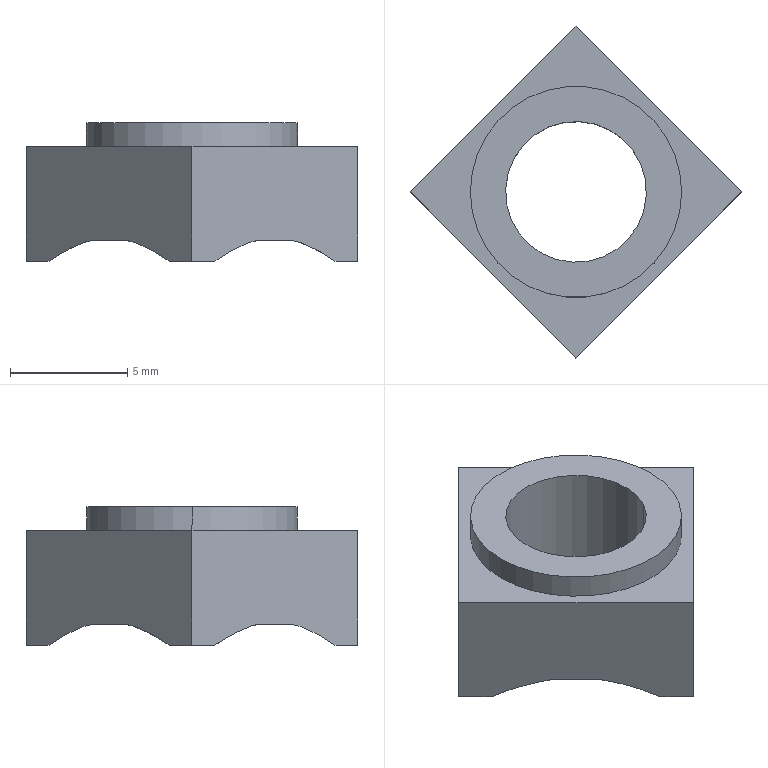Part | STEP file | Q37106 | 1 solid | 20 faces | box 14.142 x 14.142 x 5.9 mm | volume 331.042 mm3 | plane 11 | cone 5 | cylinder 4 | commonest cylinder face diameters 6 x2 9 x2
STEP:
#1=CARTESIAN_POINT('',(2.825,4.246,0.));
#2=VERTEX_POINT('',#1);
#3=CARTESIAN_POINT('',(4.246,2.825,0.));
#4=VERTEX_POINT('',#3);
#5=CARTESIAN_POINT('',(3.536,3.536,0.));
#6=DIRECTION('',(0.7071,-0.7071,0.));
#7=VECTOR('',#6,1.);
#8=LINE('',#5,#7);
#9=EDGE_CURVE('',#2,#4,#8,.T.);
#10=ORIENTED_EDGE('',*,*,#9,.T.);
#11=CARTESIAN_POINT('',(4.476,2.445,0.));
#12=VERTEX_POINT('',#11);
#13=CARTESIAN_POINT('',(0.,0.,0.));
#14=DIRECTION('',(0.,0.,1.));
#15=AXIS2_PLACEMENT_3D('',#13,#14,$);
#16=CIRCLE('',#15,5.1);
#17=EDGE_CURVE('',#12,#4,#16,.T.);
#18=ORIENTED_EDGE('',*,*,#17,.F.);
#19=CARTESIAN_POINT('',(4.246,-2.825,0.));
#20=VERTEX_POINT('',#19);
#21=CARTESIAN_POINT('',(0.,0.,0.));
#22=DIRECTION('',(0.,0.,1.));
#23=AXIS2_PLACEMENT_3D('',#21,#22,$);
#24=CIRCLE('',#23,5.1);
#25=EDGE_CURVE('',#20,#12,#24,.T.);
#26=ORIENTED_EDGE('',*,*,#25,.F.);
#27=CARTESIAN_POINT('',(2.825,-4.246,0.));
#28=VERTEX_POINT('',#27);
#29=CARTESIAN_POINT('',(3.536,-3.536,0.));
#30=DIRECTION('',(-0.7071,-0.7071,0.));
#31=VECTOR('',#30,1.);
#32=LINE('',#29,#31);
#33=EDGE_CURVE('',#20,#28,#32,.T.);
#34=ORIENTED_EDGE('',*,*,#33,.T.);
#35=CARTESIAN_POINT('',(-2.825,-4.246,0.));
#36=VERTEX_POINT('',#35);
#37=CARTESIAN_POINT('',(0.,0.,0.));
#38=DIRECTION('',(0.,0.,1.));
#39=AXIS2_PLACEMENT_3D('',#37,#38,$);
#40=CIRCLE('',#39,5.1);
#41=EDGE_CURVE('',#36,#28,#40,.T.);
#42=ORIENTED_EDGE('',*,*,#41,.F.);
#43=CARTESIAN_POINT('',(-4.246,-2.825,0.));
#44=VERTEX_POINT('',#43);
#45=CARTESIAN_POINT('',(-3.536,-3.536,0.));
#46=DIRECTION('',(0.7071,-0.7071,0.));
#47=VECTOR('',#46,1.);
#48=LINE('',#45,#47);
#49=EDGE_CURVE('',#44,#36,#48,.T.);
#50=ORIENTED_EDGE('',*,*,#49,.F.);
#51=CARTESIAN_POINT('',(-4.476,-2.445,0.));
#52=VERTEX_POINT('',#51);
#53=CARTESIAN_POINT('',(0.,0.,0.));
#54=DIRECTION('',(0.,0.,1.));
#55=AXIS2_PLACEMENT_3D('',#53,#54,$);
#56=CIRCLE('',#55,5.1);
#57=EDGE_CURVE('',#52,#44,#56,.T.);
#58=ORIENTED_EDGE('',*,*,#57,.F.);
#59=CARTESIAN_POINT('',(-4.246,2.825,0.));
#60=VERTEX_POINT('',#59);
#61=CARTESIAN_POINT('',(0.,0.,0.));
#62=DIRECTION('',(0.,0.,1.));
#63=AXIS2_PLACEMENT_3D('',#61,#62,$);
#64=CIRCLE('',#63,5.1);
#65=EDGE_CURVE('',#60,#52,#64,.T.);
#66=ORIENTED_EDGE('',*,*,#65,.F.);
#67=CARTESIAN_POINT('',(-2.825,4.246,0.));
#68=VERTEX_POINT('',#67);
#69=CARTESIAN_POINT('',(-3.536,3.536,0.));
#70=DIRECTION('',(0.7071,0.7071,0.));
#71=VECTOR('',#70,1.);
#72=LINE('',#69,#71);
#73=EDGE_CURVE('',#60,#68,#72,.T.);
#74=ORIENTED_EDGE('',*,*,#73,.T.);
#75=CARTESIAN_POINT('',(0.,0.,0.));
#76=DIRECTION('',(0.,0.,1.));
#77=AXIS2_PLACEMENT_3D('',#75,#76,$);
#78=CIRCLE('',#77,5.1);
#79=EDGE_CURVE('',#2,#68,#78,.T.);
#80=ORIENTED_EDGE('',*,*,#79,.F.);
#81=EDGE_LOOP('',(#10,#18,#26,#34,#42,#50,#58,#66,#74,#80));
#82=FACE_OUTER_BOUND('',#81,.T.);
#83=CARTESIAN_POINT('',(-2.633,1.438,0.));
#84=VERTEX_POINT('',#83);
#85=CARTESIAN_POINT('',(2.633,-1.438,0.));
#86=VERTEX_POINT('',#85);
#87=CARTESIAN_POINT('',(0.,0.,0.));
#88=DIRECTION('',(0.,0.,1.));
#89=AXIS2_PLACEMENT_3D('',#87,#88,$);
#90=CIRCLE('',#89,3.);
#91=EDGE_CURVE('',#84,#86,#90,.T.);
#92=ORIENTED_EDGE('',*,*,#91,.T.);
#93=CARTESIAN_POINT('',(0.,0.,0.));
#94=DIRECTION('',(0.,0.,1.));
#95=AXIS2_PLACEMENT_3D('',#93,#94,$);
#96=CIRCLE('',#95,3.);
#97=EDGE_CURVE('',#86,#84,#96,.T.);
#98=ORIENTED_EDGE('',*,*,#97,.T.);
#99=EDGE_LOOP('',(#92,#98));
#100=FACE_BOUND('',#99,.T.);
#101=CARTESIAN_POINT('',(0.,0.,0.));
#102=DIRECTION('',(0.,0.,1.));
#103=DIRECTION('',(1.,0.,0.));
#104=AXIS2_PLACEMENT_3D('',#101,#102,#103);
#105=PLANE('',#104);
#106=ADVANCED_FACE('',(#82,#100),#105,.F.);
#107=CARTESIAN_POINT('',(-0.9762,6.095,-0.9));
#108=VERTEX_POINT('',#107);
#109=CARTESIAN_POINT('',(-2.825,4.246,0.));
#110=CARTESIAN_POINT('',(-2.43,4.641,-0.09223));
#111=CARTESIAN_POINT('',(-2.013,5.058,-0.2568));
#112=CARTESIAN_POINT('',(-1.552,5.519,-0.4995));
#113=CARTESIAN_POINT('',(-0.9762,6.095,-0.9));
#114=B_SPLINE_CURVE_WITH_KNOTS('',4,(#109,#110,#111,#112,#113),.UNSPECIFIED.,.F.,.U.,(5,5),(0.,42.955),.UNSPECIFIED.);
#115=EDGE_CURVE('',#68,#108,#114,.T.);
#116=ORIENTED_EDGE('',*,*,#115,.T.);
#117=CARTESIAN_POINT('',(0.9762,6.095,-0.9));
#118=VERTEX_POINT('',#117);
#119=CARTESIAN_POINT('',(0.,0.,-0.9));
#120=DIRECTION('',(0.,0.,-1.));
#121=AXIS2_PLACEMENT_3D('',#119,#120,$);
#122=CIRCLE('',#121,6.173);
#123=EDGE_CURVE('',#118,#108,#122,.F.);
#124=ORIENTED_EDGE('',*,*,#123,.F.);
#125=CARTESIAN_POINT('',(2.825,4.246,0.));
#126=CARTESIAN_POINT('',(2.43,4.641,-0.09223));
#127=CARTESIAN_POINT('',(2.013,5.058,-0.2568));
#128=CARTESIAN_POINT('',(1.552,5.519,-0.4995));
#129=CARTESIAN_POINT('',(0.9762,6.095,-0.9));
#130=B_SPLINE_CURVE_WITH_KNOTS('',4,(#125,#126,#127,#128,#129),.UNSPECIFIED.,.F.,.U.,(5,5),(0.,42.955),.UNSPECIFIED.);
#131=EDGE_CURVE('',#2,#118,#130,.T.);
#132=ORIENTED_EDGE('',*,*,#131,.F.);
#133=ORIENTED_EDGE('',*,*,#79,.T.);
#134=EDGE_LOOP('',(#116,#124,#132,#133));
#135=FACE_OUTER_BOUND('',#134,.T.);
#136=CARTESIAN_POINT('',(0.,0.,0.));
#137=DIRECTION('',(0.,0.,-1.));
#138=DIRECTION('',(0.8776,0.4794,0.));
#139=AXIS2_PLACEMENT_3D('',#136,#137,#138);
#140=CONICAL_SURFACE('',#139,5.1,0.8727);
#141=ADVANCED_FACE('',(#135),#140,.F.);
#142=ORIENTED_EDGE('',*,*,#115,.F.);
#143=ORIENTED_EDGE('',*,*,#73,.F.);
#144=CARTESIAN_POINT('',(-6.095,0.9762,-0.9));
#145=VERTEX_POINT('',#144);
#146=CARTESIAN_POINT('',(-4.246,2.825,0.));
#147=CARTESIAN_POINT('',(-4.491,2.58,-0.05731));
#148=CARTESIAN_POINT('',(-4.744,2.327,-0.1403));
#149=CARTESIAN_POINT('',(-5.01,2.061,-0.2515));
#150=CARTESIAN_POINT('',(-5.378,1.693,-0.4379));
#151=CARTESIAN_POINT('',(-5.796,1.275,-0.6993));
#152=CARTESIAN_POINT('',(-5.893,1.178,-0.7617));
#153=CARTESIAN_POINT('',(-5.992,1.079,-0.8284));
#154=CARTESIAN_POINT('',(-6.095,0.9762,-0.9));
#155=B_SPLINE_CURVE_WITH_KNOTS('',5,(#146,#147,#148,#149,#150,#151,#152,#153,#154),.UNSPECIFIED.,.F.,.U.,(6,3,6),(0.,33.361,42.955),.UNSPECIFIED.);
#156=EDGE_CURVE('',#60,#145,#155,.T.);
#157=ORIENTED_EDGE('',*,*,#156,.T.);
#158=CARTESIAN_POINT('',(-7.071,0.,-0.9));
#159=VERTEX_POINT('',#158);
#160=CARTESIAN_POINT('',(-6.583,0.4881,-0.9));
#161=DIRECTION('',(0.7071,0.7071,0.));
#162=VECTOR('',#161,1.);
#163=LINE('',#160,#162);
#164=EDGE_CURVE('',#145,#159,#163,.F.);
#165=ORIENTED_EDGE('',*,*,#164,.T.);
#166=CARTESIAN_POINT('',(-7.071,0.,4.));
#167=VERTEX_POINT('',#166);
#168=CARTESIAN_POINT('',(-7.071,0.,1.55));
#169=DIRECTION('',(0.,0.,1.));
#170=VECTOR('',#169,1.);
#171=LINE('',#168,#170);
#172=EDGE_CURVE('',#159,#167,#171,.T.);
#173=ORIENTED_EDGE('',*,*,#172,.T.);
#174=CARTESIAN_POINT('',(0.,7.071,4.));
#175=VERTEX_POINT('',#174);
#176=CARTESIAN_POINT('',(-3.536,3.536,4.));
#177=DIRECTION('',(0.7071,0.7071,0.));
#178=VECTOR('',#177,1.);
#179=LINE('',#176,#178);
#180=EDGE_CURVE('',#175,#167,#179,.F.);
#181=ORIENTED_EDGE('',*,*,#180,.F.);
#182=CARTESIAN_POINT('',(0.,7.071,-0.9));
#183=VERTEX_POINT('',#182);
#184=CARTESIAN_POINT('',(0.,7.071,1.55));
#185=DIRECTION('',(0.,0.,1.));
#186=VECTOR('',#185,1.);
#187=LINE('',#184,#186);
#188=EDGE_CURVE('',#183,#175,#187,.T.);
#189=ORIENTED_EDGE('',*,*,#188,.F.);
#190=CARTESIAN_POINT('',(-0.4881,6.583,-0.9));
#191=DIRECTION('',(0.7071,0.7071,0.));
#192=VECTOR('',#191,1.);
#193=LINE('',#190,#192);
#194=EDGE_CURVE('',#183,#108,#193,.F.);
#195=ORIENTED_EDGE('',*,*,#194,.T.);
#196=EDGE_LOOP('',(#142,#143,#157,#165,#173,#181,#189,#195));
#197=FACE_OUTER_BOUND('',#196,.T.);
#198=CARTESIAN_POINT('',(-7.071,0.,0.));
#199=DIRECTION('',(0.7071,-0.7071,0.));
#200=DIRECTION('',(0.7071,0.7071,0.));
#201=AXIS2_PLACEMENT_3D('',#198,#199,#200);
#202=PLANE('',#201);
#203=ADVANCED_FACE('',(#197),#202,.F.);
#204=CARTESIAN_POINT('',(-4.573,-2.498,-0.09295));
#205=VERTEX_POINT('',#204);
#206=CARTESIAN_POINT('',(-4.246,-2.825,0.));
#207=CARTESIAN_POINT('',(-4.353,-2.718,-0.02496));
#208=CARTESIAN_POINT('',(-4.461,-2.61,-0.05574));
#209=CARTESIAN_POINT('',(-4.573,-2.498,-0.09295));
#210=B_SPLINE_CURVE_WITH_KNOTS('',3,(#206,#207,#208,#209),.UNSPECIFIED.,.F.,.U.,(4,4),(0.,8.718),.UNSPECIFIED.);
#211=EDGE_CURVE('',#44,#205,#210,.T.);
#212=ORIENTED_EDGE('',*,*,#211,.T.);
#213=CARTESIAN_POINT('',(-6.095,-0.9762,-0.9));
#214=VERTEX_POINT('',#213);
#215=CARTESIAN_POINT('',(-4.573,-2.498,-0.09295));
#216=CARTESIAN_POINT('',(-4.901,-2.17,-0.2026));
#217=CARTESIAN_POINT('',(-5.251,-1.82,-0.3625));
#218=CARTESIAN_POINT('',(-5.636,-1.435,-0.5808));
#219=CARTESIAN_POINT('',(-6.095,-0.9762,-0.9));
#220=B_SPLINE_CURVE_WITH_KNOTS('',4,(#215,#216,#217,#218,#219),.UNSPECIFIED.,.F.,.U.,(5,5),(0.,34.234),.UNSPECIFIED.);
#221=EDGE_CURVE('',#205,#214,#220,.T.);
#222=ORIENTED_EDGE('',*,*,#221,.T.);
#223=CARTESIAN_POINT('',(0.,0.,-0.9));
#224=DIRECTION('',(0.,0.,-1.));
#225=AXIS2_PLACEMENT_3D('',#223,#224,$);
#226=CIRCLE('',#225,6.173);
#227=EDGE_CURVE('',#145,#214,#226,.F.);
#228=ORIENTED_EDGE('',*,*,#227,.F.);
#229=ORIENTED_EDGE('',*,*,#156,.F.);
#230=ORIENTED_EDGE('',*,*,#65,.T.);
#231=ORIENTED_EDGE('',*,*,#57,.T.);
#232=EDGE_LOOP('',(#212,#222,#228,#229,#230,#231));
#233=FACE_OUTER_BOUND('',#232,.T.);
#234=ADVANCED_FACE('',(#233),#140,.F.);
#235=ORIENTED_EDGE('',*,*,#221,.F.);
#236=ORIENTED_EDGE('',*,*,#211,.F.);
#237=ORIENTED_EDGE('',*,*,#49,.T.);
#238=CARTESIAN_POINT('',(-0.9762,-6.095,-0.9));
#239=VERTEX_POINT('',#238);
#240=CARTESIAN_POINT('',(-2.825,-4.246,0.));
#241=CARTESIAN_POINT('',(-2.58,-4.491,-0.05731));
#242=CARTESIAN_POINT('',(-2.327,-4.744,-0.1403));
#243=CARTESIAN_POINT('',(-2.061,-5.01,-0.2515));
#244=CARTESIAN_POINT('',(-1.693,-5.378,-0.4379));
#245=CARTESIAN_POINT('',(-1.275,-5.796,-0.6993));
#246=CARTESIAN_POINT('',(-1.178,-5.893,-0.7617));
#247=CARTESIAN_POINT('',(-1.079,-5.992,-0.8284));
#248=CARTESIAN_POINT('',(-0.9762,-6.095,-0.9));
#249=B_SPLINE_CURVE_WITH_KNOTS('',5,(#240,#241,#242,#243,#244,#245,#246,#247,#248),.UNSPECIFIED.,.F.,.U.,(6,3,6),(0.,33.361,42.955),.UNSPECIFIED.);
#250=EDGE_CURVE('',#36,#239,#249,.T.);
#251=ORIENTED_EDGE('',*,*,#250,.T.);
#252=CARTESIAN_POINT('',(0.,-7.071,-0.9));
#253=VERTEX_POINT('',#252);
#254=CARTESIAN_POINT('',(-0.4881,-6.583,-0.9));
#255=DIRECTION('',(-0.7071,0.7071,0.));
#256=VECTOR('',#255,1.);
#257=LINE('',#254,#256);
#258=EDGE_CURVE('',#239,#253,#257,.F.);
#259=ORIENTED_EDGE('',*,*,#258,.T.);
#260=CARTESIAN_POINT('',(0.,-7.071,4.));
#261=VERTEX_POINT('',#260);
#262=CARTESIAN_POINT('',(0.,-7.071,1.55));
#263=DIRECTION('',(0.,0.,1.));
#264=VECTOR('',#263,1.);
#265=LINE('',#262,#264);
#266=EDGE_CURVE('',#253,#261,#265,.T.);
#267=ORIENTED_EDGE('',*,*,#266,.T.);
#268=CARTESIAN_POINT('',(-3.536,-3.536,4.));
#269=DIRECTION('',(-0.7071,0.7071,0.));
#270=VECTOR('',#269,1.);
#271=LINE('',#268,#270);
#272=EDGE_CURVE('',#167,#261,#271,.F.);
#273=ORIENTED_EDGE('',*,*,#272,.F.);
#274=ORIENTED_EDGE('',*,*,#172,.F.);
#275=CARTESIAN_POINT('',(-6.583,-0.4881,-0.9));
#276=DIRECTION('',(-0.7071,0.7071,0.));
#277=VECTOR('',#276,1.);
#278=LINE('',#275,#277);
#279=EDGE_CURVE('',#159,#214,#278,.F.);
#280=ORIENTED_EDGE('',*,*,#279,.T.);
#281=EDGE_LOOP('',(#235,#236,#237,#251,#259,#267,#273,#274,#280));
#282=FACE_OUTER_BOUND('',#281,.T.);
#283=CARTESIAN_POINT('',(0.,-7.071,0.));
#284=DIRECTION('',(0.7071,0.7071,0.));
#285=DIRECTION('',(-0.7071,0.7071,0.));
#286=AXIS2_PLACEMENT_3D('',#283,#284,#285);
#287=PLANE('',#286);
#288=ADVANCED_FACE('',(#282),#287,.F.);
#289=CARTESIAN_POINT('',(0.9762,-6.095,-0.9));
#290=VERTEX_POINT('',#289);
#291=CARTESIAN_POINT('',(2.825,-4.246,0.));
#292=CARTESIAN_POINT('',(2.43,-4.641,-0.09223));
#293=CARTESIAN_POINT('',(2.013,-5.058,-0.2568));
#294=CARTESIAN_POINT('',(1.552,-5.519,-0.4995));
#295=CARTESIAN_POINT('',(0.9762,-6.095,-0.9));
#296=B_SPLINE_CURVE_WITH_KNOTS('',4,(#291,#292,#293,#294,#295),.UNSPECIFIED.,.F.,.U.,(5,5),(0.,42.955),.UNSPECIFIED.);
#297=EDGE_CURVE('',#28,#290,#296,.T.);
#298=ORIENTED_EDGE('',*,*,#297,.T.);
#299=CARTESIAN_POINT('',(0.,0.,-0.9));
#300=DIRECTION('',(0.,0.,-1.));
#301=AXIS2_PLACEMENT_3D('',#299,#300,$);
#302=CIRCLE('',#301,6.173);
#303=EDGE_CURVE('',#239,#290,#302,.F.);
#304=ORIENTED_EDGE('',*,*,#303,.F.);
#305=ORIENTED_EDGE('',*,*,#250,.F.);
#306=ORIENTED_EDGE('',*,*,#41,.T.);
#307=EDGE_LOOP('',(#298,#304,#305,#306));
#308=FACE_OUTER_BOUND('',#307,.T.);
#309=ADVANCED_FACE('',(#308),#140,.F.);
#310=ORIENTED_EDGE('',*,*,#297,.F.);
#311=ORIENTED_EDGE('',*,*,#33,.F.);
#312=CARTESIAN_POINT('',(6.095,-0.9762,-0.9));
#313=VERTEX_POINT('',#312);
#314=CARTESIAN_POINT('',(4.246,-2.825,0.));
#315=CARTESIAN_POINT('',(4.491,-2.58,-0.05731));
#316=CARTESIAN_POINT('',(4.744,-2.327,-0.1403));
#317=CARTESIAN_POINT('',(5.01,-2.061,-0.2515));
#318=CARTESIAN_POINT('',(5.378,-1.693,-0.4379));
#319=CARTESIAN_POINT('',(5.796,-1.275,-0.6993));
#320=CARTESIAN_POINT('',(5.893,-1.178,-0.7617));
#321=CARTESIAN_POINT('',(5.992,-1.079,-0.8284));
#322=CARTESIAN_POINT('',(6.095,-0.9762,-0.9));
#323=B_SPLINE_CURVE_WITH_KNOTS('',5,(#314,#315,#316,#317,#318,#319,#320,#321,#322),.UNSPECIFIED.,.F.,.U.,(6,3,6),(0.,33.361,42.955),.UNSPECIFIED.);
#324=EDGE_CURVE('',#20,#313,#323,.T.);
#325=ORIENTED_EDGE('',*,*,#324,.T.);
#326=CARTESIAN_POINT('',(7.071,0.,-0.9));
#327=VERTEX_POINT('',#326);
#328=CARTESIAN_POINT('',(6.583,-0.4881,-0.9));
#329=DIRECTION('',(-0.7071,-0.7071,0.));
#330=VECTOR('',#329,1.);
#331=LINE('',#328,#330);
#332=EDGE_CURVE('',#313,#327,#331,.F.);
#333=ORIENTED_EDGE('',*,*,#332,.T.);
#334=CARTESIAN_POINT('',(7.071,0.,4.));
#335=VERTEX_POINT('',#334);
#336=CARTESIAN_POINT('',(7.071,0.,1.55));
#337=DIRECTION('',(0.,0.,1.));
#338=VECTOR('',#337,1.);
#339=LINE('',#336,#338);
#340=EDGE_CURVE('',#327,#335,#339,.T.);
#341=ORIENTED_EDGE('',*,*,#340,.T.);
#342=CARTESIAN_POINT('',(3.536,-3.536,4.));
#343=DIRECTION('',(-0.7071,-0.7071,0.));
#344=VECTOR('',#343,1.);
#345=LINE('',#342,#344);
#346=EDGE_CURVE('',#261,#335,#345,.F.);
#347=ORIENTED_EDGE('',*,*,#346,.F.);
#348=ORIENTED_EDGE('',*,*,#266,.F.);
#349=CARTESIAN_POINT('',(0.4881,-6.583,-0.9));
#350=DIRECTION('',(-0.7071,-0.7071,0.));
#351=VECTOR('',#350,1.);
#352=LINE('',#349,#351);
#353=EDGE_CURVE('',#253,#290,#352,.F.);
#354=ORIENTED_EDGE('',*,*,#353,.T.);
#355=EDGE_LOOP('',(#310,#311,#325,#333,#341,#347,#348,#354));
#356=FACE_OUTER_BOUND('',#355,.T.);
#357=CARTESIAN_POINT('',(7.071,0.,0.));
#358=DIRECTION('',(-0.7071,0.7071,0.));
#359=DIRECTION('',(-0.7071,-0.7071,0.));
#360=AXIS2_PLACEMENT_3D('',#357,#358,#359);
#361=PLANE('',#360);
#362=ADVANCED_FACE('',(#356),#361,.F.);
#363=CARTESIAN_POINT('',(4.573,2.498,-0.09295));
#364=VERTEX_POINT('',#363);
#365=CARTESIAN_POINT('',(6.095,0.9762,-0.9));
#366=VERTEX_POINT('',#365);
#367=CARTESIAN_POINT('',(4.573,2.498,-0.09295));
#368=CARTESIAN_POINT('',(4.901,2.17,-0.2026));
#369=CARTESIAN_POINT('',(5.251,1.82,-0.3625));
#370=CARTESIAN_POINT('',(5.636,1.435,-0.5808));
#371=CARTESIAN_POINT('',(6.095,0.9762,-0.9));
#372=B_SPLINE_CURVE_WITH_KNOTS('',4,(#367,#368,#369,#370,#371),.UNSPECIFIED.,.F.,.U.,(5,5),(0.,34.234),.UNSPECIFIED.);
#373=EDGE_CURVE('',#364,#366,#372,.T.);
#374=ORIENTED_EDGE('',*,*,#373,.T.);
#375=CARTESIAN_POINT('',(0.,0.,-0.9));
#376=DIRECTION('',(0.,0.,-1.));
#377=AXIS2_PLACEMENT_3D('',#375,#376,$);
#378=CIRCLE('',#377,6.173);
#379=EDGE_CURVE('',#313,#366,#378,.F.);
#380=ORIENTED_EDGE('',*,*,#379,.F.);
#381=ORIENTED_EDGE('',*,*,#324,.F.);
#382=ORIENTED_EDGE('',*,*,#25,.T.);
#383=CARTESIAN_POINT('',(5.014,2.739,-0.5143));
#384=DIRECTION('',(0.6723,0.3673,-0.6428));
#385=VECTOR('',#384,1.);
#386=LINE('',#383,#385);
#387=EDGE_CURVE('',#12,#364,#386,.T.);
#388=ORIENTED_EDGE('',*,*,#387,.T.);
#389=EDGE_LOOP('',(#374,#380,#381,#382,#388));
#390=FACE_OUTER_BOUND('',#389,.T.);
#391=ADVANCED_FACE('',(#390),#140,.F.);
#392=CARTESIAN_POINT('',(4.246,2.825,0.));
#393=CARTESIAN_POINT('',(4.353,2.718,-0.02496));
#394=CARTESIAN_POINT('',(4.461,2.61,-0.05574));
#395=CARTESIAN_POINT('',(4.573,2.498,-0.09295));
#396=B_SPLINE_CURVE_WITH_KNOTS('',3,(#392,#393,#394,#395),.UNSPECIFIED.,.F.,.U.,(4,4),(0.,8.718),.UNSPECIFIED.);
#397=EDGE_CURVE('',#4,#364,#396,.T.);
#398=ORIENTED_EDGE('',*,*,#397,.T.);
#399=ORIENTED_EDGE('',*,*,#387,.F.);
#400=ORIENTED_EDGE('',*,*,#17,.T.);
#401=EDGE_LOOP('',(#398,#399,#400));
#402=FACE_OUTER_BOUND('',#401,.T.);
#403=ADVANCED_FACE('',(#402),#140,.F.);
#404=ORIENTED_EDGE('',*,*,#373,.F.);
#405=ORIENTED_EDGE('',*,*,#397,.F.);
#406=ORIENTED_EDGE('',*,*,#9,.F.);
#407=ORIENTED_EDGE('',*,*,#131,.T.);
#408=CARTESIAN_POINT('',(0.4881,6.583,-0.9));
#409=DIRECTION('',(0.7071,-0.7071,0.));
#410=VECTOR('',#409,1.);
#411=LINE('',#408,#410);
#412=EDGE_CURVE('',#118,#183,#411,.F.);
#413=ORIENTED_EDGE('',*,*,#412,.T.);
#414=ORIENTED_EDGE('',*,*,#188,.T.);
#415=CARTESIAN_POINT('',(3.536,3.536,4.));
#416=DIRECTION('',(0.7071,-0.7071,0.));
#417=VECTOR('',#416,1.);
#418=LINE('',#415,#417);
#419=EDGE_CURVE('',#335,#175,#418,.F.);
#420=ORIENTED_EDGE('',*,*,#419,.F.);
#421=ORIENTED_EDGE('',*,*,#340,.F.);
#422=CARTESIAN_POINT('',(6.583,0.4881,-0.9));
#423=DIRECTION('',(0.7071,-0.7071,0.));
#424=VECTOR('',#423,1.);
#425=LINE('',#422,#424);
#426=EDGE_CURVE('',#327,#366,#425,.F.);
#427=ORIENTED_EDGE('',*,*,#426,.T.);
#428=EDGE_LOOP('',(#404,#405,#406,#407,#413,#414,#420,#421,#427));
#429=FACE_OUTER_BOUND('',#428,.T.);
#430=CARTESIAN_POINT('',(0.,7.071,0.));
#431=DIRECTION('',(-0.7071,-0.7071,0.));
#432=DIRECTION('',(0.7071,-0.7071,0.));
#433=AXIS2_PLACEMENT_3D('',#430,#431,#432);
#434=PLANE('',#433);
#435=ADVANCED_FACE('',(#429),#434,.F.);
#436=ORIENTED_EDGE('',*,*,#97,.F.);
#437=CARTESIAN_POINT('',(2.633,-1.438,5.));
#438=VERTEX_POINT('',#437);
#439=CARTESIAN_POINT('',(2.633,-1.438,2.05));
#440=DIRECTION('',(0.,0.,-1.));
#441=VECTOR('',#440,1.);
#442=LINE('',#439,#441);
#443=EDGE_CURVE('',#86,#438,#442,.F.);
#444=ORIENTED_EDGE('',*,*,#443,.T.);
#445=CARTESIAN_POINT('',(-2.633,1.438,5.));
#446=VERTEX_POINT('',#445);
#447=CARTESIAN_POINT('',(0.,0.,5.));
#448=DIRECTION('',(0.,0.,-1.));
#449=AXIS2_PLACEMENT_3D('',#447,#448,$);
#450=CIRCLE('',#449,3.);
#451=EDGE_CURVE('',#438,#446,#450,.F.);
#452=ORIENTED_EDGE('',*,*,#451,.T.);
#453=CARTESIAN_POINT('',(-2.633,1.438,2.05));
#454=DIRECTION('',(0.,0.,-1.));
#455=VECTOR('',#454,1.);
#456=LINE('',#453,#455);
#457=EDGE_CURVE('',#84,#446,#456,.F.);
#458=ORIENTED_EDGE('',*,*,#457,.F.);
#459=EDGE_LOOP('',(#436,#444,#452,#458));
#460=FACE_OUTER_BOUND('',#459,.T.);
#461=CARTESIAN_POINT('',(0.,0.,4.7));
#462=DIRECTION('',(0.,0.,-1.));
#463=DIRECTION('',(0.8776,-0.4794,0.));
#464=AXIS2_PLACEMENT_3D('',#461,#462,#463);
#465=CYLINDRICAL_SURFACE('',#464,3.);
#466=ADVANCED_FACE('',(#460),#465,.F.);
#467=ORIENTED_EDGE('',*,*,#91,.F.);
#468=ORIENTED_EDGE('',*,*,#457,.T.);
#469=CARTESIAN_POINT('',(0.,0.,5.));
#470=DIRECTION('',(0.,0.,-1.));
#471=AXIS2_PLACEMENT_3D('',#469,#470,$);
#472=CIRCLE('',#471,3.);
#473=EDGE_CURVE('',#446,#438,#472,.F.);
#474=ORIENTED_EDGE('',*,*,#473,.T.);
#475=ORIENTED_EDGE('',*,*,#443,.F.);
#476=EDGE_LOOP('',(#467,#468,#474,#475));
#477=FACE_OUTER_BOUND('',#476,.T.);
#478=ADVANCED_FACE('',(#477),#465,.F.);
#479=ORIENTED_EDGE('',*,*,#123,.T.);
#480=ORIENTED_EDGE('',*,*,#194,.F.);
#481=ORIENTED_EDGE('',*,*,#412,.F.);
#482=EDGE_LOOP('',(#479,#480,#481));
#483=FACE_OUTER_BOUND('',#482,.T.);
#484=CARTESIAN_POINT('',(0.,0.,-0.9));
#485=DIRECTION('',(0.,0.,1.));
#486=DIRECTION('',(1.,0.,0.));
#487=AXIS2_PLACEMENT_3D('',#484,#485,#486);
#488=PLANE('',#487);
#489=ADVANCED_FACE('',(#483),#488,.F.);
#490=ORIENTED_EDGE('',*,*,#227,.T.);
#491=ORIENTED_EDGE('',*,*,#279,.F.);
#492=ORIENTED_EDGE('',*,*,#164,.F.);
#493=EDGE_LOOP('',(#490,#491,#492));
#494=FACE_OUTER_BOUND('',#493,.T.);
#495=ADVANCED_FACE('',(#494),#488,.F.);
#496=ORIENTED_EDGE('',*,*,#272,.T.);
#497=ORIENTED_EDGE('',*,*,#346,.T.);
#498=ORIENTED_EDGE('',*,*,#419,.T.);
#499=ORIENTED_EDGE('',*,*,#180,.T.);
#500=EDGE_LOOP('',(#496,#497,#498,#499));
#501=FACE_OUTER_BOUND('',#500,.T.);
#502=CARTESIAN_POINT('',(4.5,0.,4.));
#503=VERTEX_POINT('',#502);
#504=CARTESIAN_POINT('',(-4.5,0.,4.));
#505=VERTEX_POINT('',#504);
#506=CARTESIAN_POINT('',(0.,0.,4.));
#507=DIRECTION('',(0.,0.,1.));
#508=AXIS2_PLACEMENT_3D('',#506,#507,$);
#509=CIRCLE('',#508,4.5);
#510=EDGE_CURVE('',#503,#505,#509,.T.);
#511=ORIENTED_EDGE('',*,*,#510,.F.);
#512=CARTESIAN_POINT('',(0.,0.,4.));
#513=DIRECTION('',(0.,0.,1.));
#514=AXIS2_PLACEMENT_3D('',#512,#513,$);
#515=CIRCLE('',#514,4.5);
#516=EDGE_CURVE('',#505,#503,#515,.T.);
#517=ORIENTED_EDGE('',*,*,#516,.F.);
#518=EDGE_LOOP('',(#511,#517));
#519=FACE_BOUND('',#518,.T.);
#520=CARTESIAN_POINT('',(0.,0.,4.));
#521=DIRECTION('',(0.,0.,1.));
#522=DIRECTION('',(1.,0.,0.));
#523=AXIS2_PLACEMENT_3D('',#520,#521,#522);
#524=PLANE('',#523);
#525=ADVANCED_FACE('',(#501,#519),#524,.T.);
#526=ORIENTED_EDGE('',*,*,#303,.T.);
#527=ORIENTED_EDGE('',*,*,#353,.F.);
#528=ORIENTED_EDGE('',*,*,#258,.F.);
#529=EDGE_LOOP('',(#526,#527,#528));
#530=FACE_OUTER_BOUND('',#529,.T.);
#531=ADVANCED_FACE('',(#530),#488,.F.);
#532=ORIENTED_EDGE('',*,*,#379,.T.);
#533=ORIENTED_EDGE('',*,*,#426,.F.);
#534=ORIENTED_EDGE('',*,*,#332,.F.);
#535=EDGE_LOOP('',(#532,#533,#534));
#536=FACE_OUTER_BOUND('',#535,.T.);
#537=ADVANCED_FACE('',(#536),#488,.F.);
#538=CARTESIAN_POINT('',(4.5,0.,5.));
#539=VERTEX_POINT('',#538);
#540=CARTESIAN_POINT('',(-4.5,0.,5.));
#541=VERTEX_POINT('',#540);
#542=CARTESIAN_POINT('',(0.,0.,5.));
#543=DIRECTION('',(0.,0.,1.));
#544=AXIS2_PLACEMENT_3D('',#542,#543,$);
#545=CIRCLE('',#544,4.5);
#546=EDGE_CURVE('',#539,#541,#545,.T.);
#547=ORIENTED_EDGE('',*,*,#546,.T.);
#548=CARTESIAN_POINT('',(0.,0.,5.));
#549=DIRECTION('',(0.,0.,1.));
#550=AXIS2_PLACEMENT_3D('',#548,#549,$);
#551=CIRCLE('',#550,4.5);
#552=EDGE_CURVE('',#541,#539,#551,.T.);
#553=ORIENTED_EDGE('',*,*,#552,.T.);
#554=EDGE_LOOP('',(#547,#553));
#555=FACE_OUTER_BOUND('',#554,.T.);
#556=ORIENTED_EDGE('',*,*,#473,.F.);
#557=ORIENTED_EDGE('',*,*,#451,.F.);
#558=EDGE_LOOP('',(#556,#557));
#559=FACE_BOUND('',#558,.T.);
#560=CARTESIAN_POINT('',(0.,0.,5.));
#561=DIRECTION('',(0.,0.,1.));
#562=DIRECTION('',(1.,0.,0.));
#563=AXIS2_PLACEMENT_3D('',#560,#561,#562);
#564=PLANE('',#563);
#565=ADVANCED_FACE('',(#555,#559),#564,.T.);
#566=CARTESIAN_POINT('',(4.5,0.,4.5));
#567=DIRECTION('',(0.,0.,1.));
#568=VECTOR('',#567,1.);
#569=LINE('',#566,#568);
#570=EDGE_CURVE('',#503,#539,#569,.T.);
#571=ORIENTED_EDGE('',*,*,#570,.F.);
#572=ORIENTED_EDGE('',*,*,#510,.T.);
#573=CARTESIAN_POINT('',(-4.5,0.,4.5));
#574=DIRECTION('',(0.,0.,1.));
#575=VECTOR('',#574,1.);
#576=LINE('',#573,#575);
#577=EDGE_CURVE('',#505,#541,#576,.T.);
#578=ORIENTED_EDGE('',*,*,#577,.T.);
#579=ORIENTED_EDGE('',*,*,#546,.F.);
#580=EDGE_LOOP('',(#571,#572,#578,#579));
#581=FACE_OUTER_BOUND('',#580,.T.);
#582=CARTESIAN_POINT('',(0.,0.,4.5));
#583=DIRECTION('',(0.,0.,1.));
#584=DIRECTION('',(1.,0.,0.));
#585=AXIS2_PLACEMENT_3D('',#582,#583,#584);
#586=CYLINDRICAL_SURFACE('',#585,4.5);
#587=ADVANCED_FACE('',(#581),#586,.T.);
#588=ORIENTED_EDGE('',*,*,#577,.F.);
#589=ORIENTED_EDGE('',*,*,#516,.T.);
#590=ORIENTED_EDGE('',*,*,#570,.T.);
#591=ORIENTED_EDGE('',*,*,#552,.F.);
#592=EDGE_LOOP('',(#588,#589,#590,#591));
#593=FACE_OUTER_BOUND('',#592,.T.);
#594=ADVANCED_FACE('',(#593),#586,.T.);
#595=CLOSED_SHELL('',(#106,#141,#203,#234,#288,#309,#362,#391,#403,#435,#466,#478,#489,#495,#525,#531,#537,#565,#587,#594));
#596=MANIFOLD_SOLID_BREP('',#595);
#597=(LENGTH_UNIT()NAMED_UNIT(*)SI_UNIT(.MILLI.,.METRE.));
#598=UNCERTAINTY_MEASURE_WITH_UNIT(LENGTH_MEASURE(0.005),#597,'','');
#599=(NAMED_UNIT(*)PLANE_ANGLE_UNIT()SI_UNIT($,.RADIAN.));
#600=(NAMED_UNIT(*)SI_UNIT($,.STERADIAN.)SOLID_ANGLE_UNIT());
#601=(GEOMETRIC_REPRESENTATION_CONTEXT(3)GLOBAL_UNCERTAINTY_ASSIGNED_CONTEXT((#598))GLOBAL_UNIT_ASSIGNED_CONTEXT((#597,#599,#600))REPRESENTATION_CONTEXT('',''));
#602=ADVANCED_BREP_SHAPE_REPRESENTATION('',(#596),#601);